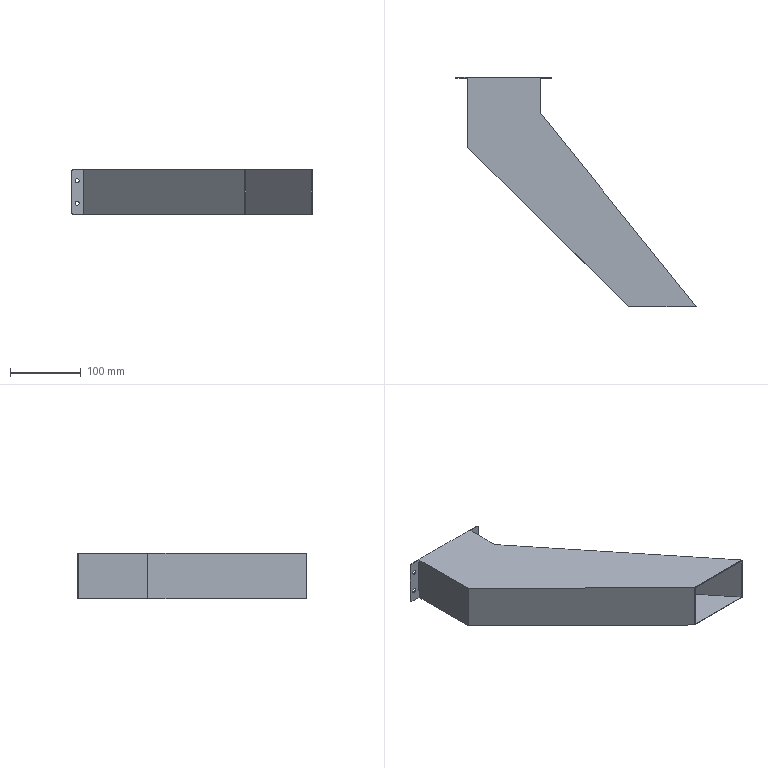Part | NX | 1 solid | 30 faces | box 340.79 x 325 x 65 mm | volume 130070 mm3 | plane 18 | cylinder 12 | commonest cylinder face diameters 6 x12
STEP:
#1=CARTESIAN_POINT('',(621.,-133.5,-79.28));
#2=VERTEX_POINT('',#1);
#3=CARTESIAN_POINT('',(607.526,-133.5,-79.28));
#4=VERTEX_POINT('',#3);
#5=CARTESIAN_POINT('',(556.,-133.5,-79.28));
#6=DIRECTION('',(-1.,0.,0.));
#7=VECTOR('',#6,1000.);
#8=LINE('',#5,#7);
#9=EDGE_CURVE('',#2,#4,#8,.T.);
#10=ORIENTED_EDGE('',*,*,#9,.T.);
#11=CARTESIAN_POINT('',(607.526,-133.5,-144.28));
#12=VERTEX_POINT('',#11);
#13=CARTESIAN_POINT('',(607.526,-133.5,-79.28));
#14=DIRECTION('',(0.,0.,-1.));
#15=VECTOR('',#14,1000.);
#16=LINE('',#13,#15);
#17=EDGE_CURVE('',#4,#12,#16,.T.);
#18=ORIENTED_EDGE('',*,*,#17,.T.);
#19=CARTESIAN_POINT('',(621.,-133.5,-144.28));
#20=VERTEX_POINT('',#19);
#21=CARTESIAN_POINT('',(556.,-133.5,-144.28));
#22=DIRECTION('',(-1.,0.,0.));
#23=VECTOR('',#22,1000.);
#24=LINE('',#21,#23);
#25=EDGE_CURVE('',#20,#12,#24,.T.);
#26=ORIENTED_EDGE('',*,*,#25,.F.);
#27=CARTESIAN_POINT('',(624.,-133.5,-141.28));
#28=VERTEX_POINT('',#27);
#29=CARTESIAN_POINT('',(621.,-133.5,-141.28));
#30=DIRECTION('',(0.,-1.,0.));
#31=DIRECTION('',(-1.,0.,0.));
#32=AXIS2_PLACEMENT_3D('',#29,#30,#31);
#33=CIRCLE('',#32,3.);
#34=EDGE_CURVE('',#20,#28,#33,.T.);
#35=ORIENTED_EDGE('',*,*,#34,.T.);
#36=CARTESIAN_POINT('',(624.,-133.5,-82.28));
#37=VERTEX_POINT('',#36);
#38=CARTESIAN_POINT('',(624.,-133.5,-79.28));
#39=DIRECTION('',(0.,0.,-1.));
#40=VECTOR('',#39,1000.);
#41=LINE('',#38,#40);
#42=EDGE_CURVE('',#37,#28,#41,.T.);
#43=ORIENTED_EDGE('',*,*,#42,.F.);
#44=CARTESIAN_POINT('',(621.,-133.5,-82.28));
#45=DIRECTION('',(0.,-1.,0.));
#46=DIRECTION('',(-1.,0.,0.));
#47=AXIS2_PLACEMENT_3D('',#44,#45,#46);
#48=CIRCLE('',#47,3.);
#49=EDGE_CURVE('',#37,#2,#48,.T.);
#50=ORIENTED_EDGE('',*,*,#49,.T.);
#51=EDGE_LOOP('',(#10,#18,#26,#35,#43,#50));
#52=FACE_BOUND('',#51,.T.);
#53=CARTESIAN_POINT('',(619.5,-133.5,-96.03));
#54=VERTEX_POINT('',#53);
#55=CARTESIAN_POINT('',(613.5,-133.5,-96.03));
#56=VERTEX_POINT('',#55);
#57=CARTESIAN_POINT('',(616.5,-133.5,-96.03));
#58=DIRECTION('',(0.,-1.,0.));
#59=DIRECTION('',(-1.,0.,0.));
#60=AXIS2_PLACEMENT_3D('',#57,#58,#59);
#61=CIRCLE('',#60,3.);
#62=EDGE_CURVE('',#54,#56,#61,.T.);
#63=ORIENTED_EDGE('',*,*,#62,.F.);
#64=CARTESIAN_POINT('',(616.5,-133.5,-96.03));
#65=DIRECTION('',(0.,-1.,0.));
#66=DIRECTION('',(-1.,0.,0.));
#67=AXIS2_PLACEMENT_3D('',#64,#65,#66);
#68=CIRCLE('',#67,3.);
#69=EDGE_CURVE('',#56,#54,#68,.T.);
#70=ORIENTED_EDGE('',*,*,#69,.F.);
#71=EDGE_LOOP('',(#63,#70));
#72=FACE_BOUND('',#71,.T.);
#73=CARTESIAN_POINT('',(619.5,-133.5,-127.53));
#74=VERTEX_POINT('',#73);
#75=CARTESIAN_POINT('',(613.5,-133.5,-127.53));
#76=VERTEX_POINT('',#75);
#77=CARTESIAN_POINT('',(616.5,-133.5,-127.53));
#78=DIRECTION('',(0.,-1.,0.));
#79=DIRECTION('',(-1.,0.,0.));
#80=AXIS2_PLACEMENT_3D('',#77,#78,#79);
#81=CIRCLE('',#80,3.);
#82=EDGE_CURVE('',#74,#76,#81,.T.);
#83=ORIENTED_EDGE('',*,*,#82,.F.);
#84=CARTESIAN_POINT('',(616.5,-133.5,-127.53));
#85=DIRECTION('',(0.,-1.,0.));
#86=DIRECTION('',(-1.,0.,0.));
#87=AXIS2_PLACEMENT_3D('',#84,#85,#86);
#88=CIRCLE('',#87,3.);
#89=EDGE_CURVE('',#76,#74,#88,.T.);
#90=ORIENTED_EDGE('',*,*,#89,.F.);
#91=EDGE_LOOP('',(#83,#90));
#92=FACE_BOUND('',#91,.T.);
#93=CARTESIAN_POINT('',(607.526,-133.5,-79.28));
#94=DIRECTION('',(0.,-1.,0.));
#95=DIRECTION('',(0.,0.,-1.));
#96=AXIS2_PLACEMENT_3D('',#93,#94,#95);
#97=PLANE('',#96);
#98=ADVANCED_FACE('',(#52,#72,#92),#97,.T.);
#99=CARTESIAN_POINT('',(607.526,-182.5,-79.28));
#100=VERTEX_POINT('',#99);
#101=CARTESIAN_POINT('',(607.526,-132.5,-79.28));
#102=DIRECTION('',(0.,-1.,0.));
#103=VECTOR('',#102,1000.);
#104=LINE('',#101,#103);
#105=EDGE_CURVE('',#4,#100,#104,.T.);
#106=ORIENTED_EDGE('',*,*,#105,.T.);
#107=CARTESIAN_POINT('',(607.526,-182.5,-144.28));
#108=VERTEX_POINT('',#107);
#109=CARTESIAN_POINT('',(607.526,-182.5,-79.28));
#110=DIRECTION('',(0.,0.,-1.));
#111=VECTOR('',#110,1000.);
#112=LINE('',#109,#111);
#113=EDGE_CURVE('',#100,#108,#112,.T.);
#114=ORIENTED_EDGE('',*,*,#113,.T.);
#115=CARTESIAN_POINT('',(607.526,-132.5,-144.28));
#116=DIRECTION('',(0.,-1.,0.));
#117=VECTOR('',#116,1000.);
#118=LINE('',#115,#117);
#119=EDGE_CURVE('',#12,#108,#118,.T.);
#120=ORIENTED_EDGE('',*,*,#119,.F.);
#121=ORIENTED_EDGE('',*,*,#17,.F.);
#122=EDGE_LOOP('',(#106,#114,#120,#121));
#123=FACE_BOUND('',#122,.T.);
#124=CARTESIAN_POINT('',(607.526,-182.5,-79.28));
#125=DIRECTION('',(1.,0.,0.));
#126=DIRECTION('',(0.,1.,0.));
#127=AXIS2_PLACEMENT_3D('',#124,#125,#126);
#128=PLANE('',#127);
#129=ADVANCED_FACE('',(#123),#128,.T.);
#130=CARTESIAN_POINT('',(828.79,-457.5,-79.28));
#131=VERTEX_POINT('',#130);
#132=CARTESIAN_POINT('',(466.156,-6.797,-79.28));
#133=DIRECTION('',(0.6269,-0.7791,0.));
#134=VECTOR('',#133,1000.);
#135=LINE('',#132,#134);
#136=EDGE_CURVE('',#100,#131,#135,.T.);
#137=ORIENTED_EDGE('',*,*,#136,.T.);
#138=CARTESIAN_POINT('',(828.79,-457.5,-144.28));
#139=VERTEX_POINT('',#138);
#140=CARTESIAN_POINT('',(828.79,-457.5,-79.28));
#141=DIRECTION('',(0.,0.,-1.));
#142=VECTOR('',#141,1000.);
#143=LINE('',#140,#142);
#144=EDGE_CURVE('',#131,#139,#143,.T.);
#145=ORIENTED_EDGE('',*,*,#144,.T.);
#146=CARTESIAN_POINT('',(466.156,-6.797,-144.28));
#147=DIRECTION('',(0.6269,-0.7791,0.));
#148=VECTOR('',#147,1000.);
#149=LINE('',#146,#148);
#150=EDGE_CURVE('',#108,#139,#149,.T.);
#151=ORIENTED_EDGE('',*,*,#150,.F.);
#152=ORIENTED_EDGE('',*,*,#113,.F.);
#153=EDGE_LOOP('',(#137,#145,#151,#152));
#154=FACE_BOUND('',#153,.T.);
#155=CARTESIAN_POINT('',(828.79,-457.5,-79.28));
#156=DIRECTION('',(0.7791,0.6269,0.));
#157=DIRECTION('',(0.,0.,-1.));
#158=AXIS2_PLACEMENT_3D('',#155,#156,#157);
#159=PLANE('',#158);
#160=ADVANCED_FACE('',(#154),#159,.T.);
#161=CARTESIAN_POINT('',(733.247,-457.5,-79.28));
#162=VERTEX_POINT('',#161);
#163=CARTESIAN_POINT('',(564.98,-457.5,-79.28));
#164=DIRECTION('',(1.,0.,0.));
#165=VECTOR('',#164,1000.);
#166=LINE('',#163,#165);
#167=EDGE_CURVE('',#162,#131,#166,.T.);
#168=ORIENTED_EDGE('',*,*,#167,.F.);
#169=CARTESIAN_POINT('',(733.247,-457.5,-144.28));
#170=VERTEX_POINT('',#169);
#171=CARTESIAN_POINT('',(733.247,-457.5,-79.28));
#172=DIRECTION('',(0.,0.,-1.));
#173=VECTOR('',#172,1000.);
#174=LINE('',#171,#173);
#175=EDGE_CURVE('',#162,#170,#174,.T.);
#176=ORIENTED_EDGE('',*,*,#175,.T.);
#177=CARTESIAN_POINT('',(564.98,-457.5,-144.28));
#178=DIRECTION('',(1.,0.,0.));
#179=VECTOR('',#178,1000.);
#180=LINE('',#177,#179);
#181=EDGE_CURVE('',#170,#139,#180,.T.);
#182=ORIENTED_EDGE('',*,*,#181,.T.);
#183=ORIENTED_EDGE('',*,*,#144,.F.);
#184=EDGE_LOOP('',(#168,#176,#182,#183));
#185=FACE_BOUND('',#184,.T.);
#186=CARTESIAN_POINT('',(734.672,-457.5,-80.28));
#187=VERTEX_POINT('',#186);
#188=CARTESIAN_POINT('',(734.672,-457.5,-143.28));
#189=VERTEX_POINT('',#188);
#190=CARTESIAN_POINT('',(734.672,-457.5,-79.28));
#191=DIRECTION('',(0.,0.,-1.));
#192=VECTOR('',#191,1000.);
#193=LINE('',#190,#192);
#194=EDGE_CURVE('',#187,#189,#193,.T.);
#195=ORIENTED_EDGE('',*,*,#194,.F.);
#196=CARTESIAN_POINT('',(827.507,-457.5,-80.28));
#197=VERTEX_POINT('',#196);
#198=CARTESIAN_POINT('',(1140.033,-457.5,-80.28));
#199=DIRECTION('',(-1.,0.,0.));
#200=VECTOR('',#199,1000.);
#201=LINE('',#198,#200);
#202=EDGE_CURVE('',#197,#187,#201,.T.);
#203=ORIENTED_EDGE('',*,*,#202,.F.);
#204=CARTESIAN_POINT('',(827.507,-457.5,-143.28));
#205=VERTEX_POINT('',#204);
#206=CARTESIAN_POINT('',(827.507,-457.5,-79.28));
#207=DIRECTION('',(0.,0.,1.));
#208=VECTOR('',#207,1000.);
#209=LINE('',#206,#208);
#210=EDGE_CURVE('',#205,#197,#209,.T.);
#211=ORIENTED_EDGE('',*,*,#210,.F.);
#212=CARTESIAN_POINT('',(1140.033,-457.5,-143.28));
#213=DIRECTION('',(-1.,0.,0.));
#214=VECTOR('',#213,1000.);
#215=LINE('',#212,#214);
#216=EDGE_CURVE('',#205,#189,#215,.T.);
#217=ORIENTED_EDGE('',*,*,#216,.T.);
#218=EDGE_LOOP('',(#195,#203,#211,#217));
#219=FACE_BOUND('',#218,.T.);
#220=CARTESIAN_POINT('',(733.247,-457.5,-79.28));
#221=DIRECTION('',(0.,-1.,0.));
#222=DIRECTION('',(0.,0.,-1.));
#223=AXIS2_PLACEMENT_3D('',#220,#221,#222);
#224=PLANE('',#223);
#225=ADVANCED_FACE('',(#185,#219),#224,.T.);
#226=CARTESIAN_POINT('',(505.,-232.5,-79.28));
#227=VERTEX_POINT('',#226);
#228=CARTESIAN_POINT('',(564.98,-291.626,-79.28));
#229=DIRECTION('',(-0.7122,0.702,0.));
#230=VECTOR('',#229,1000.);
#231=LINE('',#228,#230);
#232=EDGE_CURVE('',#162,#227,#231,.T.);
#233=ORIENTED_EDGE('',*,*,#232,.T.);
#234=CARTESIAN_POINT('',(505.,-232.5,-144.28));
#235=VERTEX_POINT('',#234);
#236=CARTESIAN_POINT('',(505.,-232.5,-79.28));
#237=DIRECTION('',(0.,0.,-1.));
#238=VECTOR('',#237,1000.);
#239=LINE('',#236,#238);
#240=EDGE_CURVE('',#227,#235,#239,.T.);
#241=ORIENTED_EDGE('',*,*,#240,.T.);
#242=CARTESIAN_POINT('',(564.98,-291.626,-144.28));
#243=DIRECTION('',(-0.7122,0.702,0.));
#244=VECTOR('',#243,1000.);
#245=LINE('',#242,#244);
#246=EDGE_CURVE('',#170,#235,#245,.T.);
#247=ORIENTED_EDGE('',*,*,#246,.F.);
#248=ORIENTED_EDGE('',*,*,#175,.F.);
#249=EDGE_LOOP('',(#233,#241,#247,#248));
#250=FACE_BOUND('',#249,.T.);
#251=CARTESIAN_POINT('',(505.,-232.5,-79.28));
#252=DIRECTION('',(-0.702,-0.7122,0.));
#253=DIRECTION('',(-0.7122,0.702,0.));
#254=AXIS2_PLACEMENT_3D('',#251,#252,#253);
#255=PLANE('',#254);
#256=ADVANCED_FACE('',(#250),#255,.T.);
#257=CARTESIAN_POINT('',(505.,-133.5,-79.28));
#258=VERTEX_POINT('',#257);
#259=CARTESIAN_POINT('',(505.,-132.5,-79.28));
#260=DIRECTION('',(0.,-1.,0.));
#261=VECTOR('',#260,1000.);
#262=LINE('',#259,#261);
#263=EDGE_CURVE('',#258,#227,#262,.T.);
#264=ORIENTED_EDGE('',*,*,#263,.F.);
#265=CARTESIAN_POINT('',(505.,-133.5,-144.28));
#266=VERTEX_POINT('',#265);
#267=CARTESIAN_POINT('',(505.,-133.5,-79.28));
#268=DIRECTION('',(0.,0.,-1.));
#269=VECTOR('',#268,1000.);
#270=LINE('',#267,#269);
#271=EDGE_CURVE('',#258,#266,#270,.T.);
#272=ORIENTED_EDGE('',*,*,#271,.T.);
#273=CARTESIAN_POINT('',(505.,-132.5,-144.28));
#274=DIRECTION('',(0.,-1.,0.));
#275=VECTOR('',#274,1000.);
#276=LINE('',#273,#275);
#277=EDGE_CURVE('',#266,#235,#276,.T.);
#278=ORIENTED_EDGE('',*,*,#277,.T.);
#279=ORIENTED_EDGE('',*,*,#240,.F.);
#280=EDGE_LOOP('',(#264,#272,#278,#279));
#281=FACE_BOUND('',#280,.T.);
#282=CARTESIAN_POINT('',(505.,-133.5,-79.28));
#283=DIRECTION('',(-1.,0.,0.));
#284=DIRECTION('',(0.,1.,0.));
#285=AXIS2_PLACEMENT_3D('',#282,#283,#284);
#286=PLANE('',#285);
#287=ADVANCED_FACE('',(#281),#286,.T.);
#288=CARTESIAN_POINT('',(491.,-133.5,-79.28));
#289=VERTEX_POINT('',#288);
#290=CARTESIAN_POINT('',(556.,-133.5,-79.28));
#291=DIRECTION('',(-1.,0.,0.));
#292=VECTOR('',#291,1000.);
#293=LINE('',#290,#292);
#294=EDGE_CURVE('',#258,#289,#293,.T.);
#295=ORIENTED_EDGE('',*,*,#294,.T.);
#296=CARTESIAN_POINT('',(488.,-133.5,-82.28));
#297=VERTEX_POINT('',#296);
#298=CARTESIAN_POINT('',(491.,-133.5,-82.28));
#299=DIRECTION('',(0.,-1.,0.));
#300=DIRECTION('',(-1.,0.,0.));
#301=AXIS2_PLACEMENT_3D('',#298,#299,#300);
#302=CIRCLE('',#301,3.);
#303=EDGE_CURVE('',#289,#297,#302,.T.);
#304=ORIENTED_EDGE('',*,*,#303,.T.);
#305=CARTESIAN_POINT('',(488.,-133.5,-141.28));
#306=VERTEX_POINT('',#305);
#307=CARTESIAN_POINT('',(488.,-133.5,-79.28));
#308=DIRECTION('',(0.,0.,-1.));
#309=VECTOR('',#308,1000.);
#310=LINE('',#307,#309);
#311=EDGE_CURVE('',#297,#306,#310,.T.);
#312=ORIENTED_EDGE('',*,*,#311,.T.);
#313=CARTESIAN_POINT('',(491.,-133.5,-144.28));
#314=VERTEX_POINT('',#313);
#315=CARTESIAN_POINT('',(491.,-133.5,-141.28));
#316=DIRECTION('',(0.,-1.,0.));
#317=DIRECTION('',(-1.,0.,0.));
#318=AXIS2_PLACEMENT_3D('',#315,#316,#317);
#319=CIRCLE('',#318,3.);
#320=EDGE_CURVE('',#306,#314,#319,.T.);
#321=ORIENTED_EDGE('',*,*,#320,.T.);
#322=CARTESIAN_POINT('',(556.,-133.5,-144.28));
#323=DIRECTION('',(-1.,0.,0.));
#324=VECTOR('',#323,1000.);
#325=LINE('',#322,#324);
#326=EDGE_CURVE('',#266,#314,#325,.T.);
#327=ORIENTED_EDGE('',*,*,#326,.F.);
#328=ORIENTED_EDGE('',*,*,#271,.F.);
#329=EDGE_LOOP('',(#295,#304,#312,#321,#327,#328));
#330=FACE_BOUND('',#329,.T.);
#331=CARTESIAN_POINT('',(498.5,-133.5,-96.03));
#332=VERTEX_POINT('',#331);
#333=CARTESIAN_POINT('',(492.5,-133.5,-96.03));
#334=VERTEX_POINT('',#333);
#335=CARTESIAN_POINT('',(495.5,-133.5,-96.03));
#336=DIRECTION('',(0.,-1.,0.));
#337=DIRECTION('',(-1.,0.,0.));
#338=AXIS2_PLACEMENT_3D('',#335,#336,#337);
#339=CIRCLE('',#338,3.);
#340=EDGE_CURVE('',#332,#334,#339,.T.);
#341=ORIENTED_EDGE('',*,*,#340,.F.);
#342=CARTESIAN_POINT('',(495.5,-133.5,-96.03));
#343=DIRECTION('',(0.,-1.,0.));
#344=DIRECTION('',(-1.,0.,0.));
#345=AXIS2_PLACEMENT_3D('',#342,#343,#344);
#346=CIRCLE('',#345,3.);
#347=EDGE_CURVE('',#334,#332,#346,.T.);
#348=ORIENTED_EDGE('',*,*,#347,.F.);
#349=EDGE_LOOP('',(#341,#348));
#350=FACE_BOUND('',#349,.T.);
#351=CARTESIAN_POINT('',(498.5,-133.5,-127.53));
#352=VERTEX_POINT('',#351);
#353=CARTESIAN_POINT('',(492.5,-133.5,-127.53));
#354=VERTEX_POINT('',#353);
#355=CARTESIAN_POINT('',(495.5,-133.5,-127.53));
#356=DIRECTION('',(0.,-1.,0.));
#357=DIRECTION('',(-1.,0.,0.));
#358=AXIS2_PLACEMENT_3D('',#355,#356,#357);
#359=CIRCLE('',#358,3.);
#360=EDGE_CURVE('',#352,#354,#359,.T.);
#361=ORIENTED_EDGE('',*,*,#360,.F.);
#362=CARTESIAN_POINT('',(495.5,-133.5,-127.53));
#363=DIRECTION('',(0.,-1.,0.));
#364=DIRECTION('',(-1.,0.,0.));
#365=AXIS2_PLACEMENT_3D('',#362,#363,#364);
#366=CIRCLE('',#365,3.);
#367=EDGE_CURVE('',#354,#352,#366,.T.);
#368=ORIENTED_EDGE('',*,*,#367,.F.);
#369=EDGE_LOOP('',(#361,#368));
#370=FACE_BOUND('',#369,.T.);
#371=CARTESIAN_POINT('',(488.,-133.5,-79.28));
#372=DIRECTION('',(0.,-1.,0.));
#373=DIRECTION('',(0.,0.,-1.));
#374=AXIS2_PLACEMENT_3D('',#371,#372,#373);
#375=PLANE('',#374);
#376=ADVANCED_FACE('',(#330,#350,#370),#375,.T.);
#377=CARTESIAN_POINT('',(488.,-132.5,-82.28));
#378=VERTEX_POINT('',#377);
#379=CARTESIAN_POINT('',(488.,-72.544,-82.28));
#380=DIRECTION('',(0.,-1.,0.));
#381=VECTOR('',#380,1000.);
#382=LINE('',#379,#381);
#383=EDGE_CURVE('',#378,#297,#382,.T.);
#384=ORIENTED_EDGE('',*,*,#383,.F.);
#385=CARTESIAN_POINT('',(488.,-132.5,-141.28));
#386=VERTEX_POINT('',#385);
#387=CARTESIAN_POINT('',(488.,-132.5,-79.28));
#388=DIRECTION('',(0.,0.,-1.));
#389=VECTOR('',#388,1000.);
#390=LINE('',#387,#389);
#391=EDGE_CURVE('',#378,#386,#390,.T.);
#392=ORIENTED_EDGE('',*,*,#391,.T.);
#393=CARTESIAN_POINT('',(488.,-72.544,-141.28));
#394=DIRECTION('',(0.,-1.,0.));
#395=VECTOR('',#394,1000.);
#396=LINE('',#393,#395);
#397=EDGE_CURVE('',#386,#306,#396,.T.);
#398=ORIENTED_EDGE('',*,*,#397,.T.);
#399=ORIENTED_EDGE('',*,*,#311,.F.);
#400=EDGE_LOOP('',(#384,#392,#398,#399));
#401=FACE_BOUND('',#400,.T.);
#402=CARTESIAN_POINT('',(488.,-132.5,-79.28));
#403=DIRECTION('',(-1.,0.,0.));
#404=DIRECTION('',(0.,0.,1.));
#405=AXIS2_PLACEMENT_3D('',#402,#403,#404);
#406=PLANE('',#405);
#407=ADVANCED_FACE('',(#401),#406,.T.);
#408=CARTESIAN_POINT('',(621.,-132.5,-79.28));
#409=VERTEX_POINT('',#408);
#410=CARTESIAN_POINT('',(491.,-132.5,-79.28));
#411=VERTEX_POINT('',#410);
#412=CARTESIAN_POINT('',(556.,-132.5,-79.28));
#413=DIRECTION('',(-1.,0.,0.));
#414=VECTOR('',#413,1000.);
#415=LINE('',#412,#414);
#416=EDGE_CURVE('',#409,#411,#415,.T.);
#417=ORIENTED_EDGE('',*,*,#416,.F.);
#418=CARTESIAN_POINT('',(624.,-132.5,-82.28));
#419=VERTEX_POINT('',#418);
#420=CARTESIAN_POINT('',(621.,-132.5,-82.28));
#421=DIRECTION('',(0.,-1.,0.));
#422=DIRECTION('',(-1.,0.,0.));
#423=AXIS2_PLACEMENT_3D('',#420,#421,#422);
#424=CIRCLE('',#423,3.);
#425=EDGE_CURVE('',#419,#409,#424,.T.);
#426=ORIENTED_EDGE('',*,*,#425,.F.);
#427=CARTESIAN_POINT('',(624.,-132.5,-141.28));
#428=VERTEX_POINT('',#427);
#429=CARTESIAN_POINT('',(624.,-132.5,-79.28));
#430=DIRECTION('',(0.,0.,-1.));
#431=VECTOR('',#430,1000.);
#432=LINE('',#429,#431);
#433=EDGE_CURVE('',#419,#428,#432,.T.);
#434=ORIENTED_EDGE('',*,*,#433,.T.);
#435=CARTESIAN_POINT('',(621.,-132.5,-144.28));
#436=VERTEX_POINT('',#435);
#437=CARTESIAN_POINT('',(621.,-132.5,-141.28));
#438=DIRECTION('',(0.,-1.,0.));
#439=DIRECTION('',(-1.,0.,0.));
#440=AXIS2_PLACEMENT_3D('',#437,#438,#439);
#441=CIRCLE('',#440,3.);
#442=EDGE_CURVE('',#436,#428,#441,.T.);
#443=ORIENTED_EDGE('',*,*,#442,.F.);
#444=CARTESIAN_POINT('',(491.,-132.5,-144.28));
#445=VERTEX_POINT('',#444);
#446=CARTESIAN_POINT('',(556.,-132.5,-144.28));
#447=DIRECTION('',(-1.,0.,0.));
#448=VECTOR('',#447,1000.);
#449=LINE('',#446,#448);
#450=EDGE_CURVE('',#436,#445,#449,.T.);
#451=ORIENTED_EDGE('',*,*,#450,.T.);
#452=CARTESIAN_POINT('',(491.,-132.5,-141.28));
#453=DIRECTION('',(0.,-1.,0.));
#454=DIRECTION('',(-1.,0.,0.));
#455=AXIS2_PLACEMENT_3D('',#452,#453,#454);
#456=CIRCLE('',#455,3.);
#457=EDGE_CURVE('',#386,#445,#456,.T.);
#458=ORIENTED_EDGE('',*,*,#457,.F.);
#459=ORIENTED_EDGE('',*,*,#391,.F.);
#460=CARTESIAN_POINT('',(491.,-132.5,-82.28));
#461=DIRECTION('',(0.,-1.,0.));
#462=DIRECTION('',(-1.,0.,0.));
#463=AXIS2_PLACEMENT_3D('',#460,#461,#462);
#464=CIRCLE('',#463,3.);
#465=EDGE_CURVE('',#411,#378,#464,.T.);
#466=ORIENTED_EDGE('',*,*,#465,.F.);
#467=EDGE_LOOP('',(#417,#426,#434,#443,#451,#458,#459,#466));
#468=FACE_BOUND('',#467,.T.);
#469=CARTESIAN_POINT('',(506.,-132.5,-143.28));
#470=VERTEX_POINT('',#469);
#471=CARTESIAN_POINT('',(506.,-132.5,-80.28));
#472=VERTEX_POINT('',#471);
#473=CARTESIAN_POINT('',(506.,-132.5,-79.28));
#474=DIRECTION('',(0.,0.,1.));
#475=VECTOR('',#474,1000.);
#476=LINE('',#473,#475);
#477=EDGE_CURVE('',#470,#472,#476,.T.);
#478=ORIENTED_EDGE('',*,*,#477,.F.);
#479=CARTESIAN_POINT('',(606.526,-132.5,-143.28));
#480=VERTEX_POINT('',#479);
#481=CARTESIAN_POINT('',(1140.033,-132.5,-143.28));
#482=DIRECTION('',(-1.,0.,0.));
#483=VECTOR('',#482,1000.);
#484=LINE('',#481,#483);
#485=EDGE_CURVE('',#480,#470,#484,.T.);
#486=ORIENTED_EDGE('',*,*,#485,.F.);
#487=CARTESIAN_POINT('',(606.526,-132.5,-80.28));
#488=VERTEX_POINT('',#487);
#489=CARTESIAN_POINT('',(606.526,-132.5,-79.28));
#490=DIRECTION('',(0.,0.,-1.));
#491=VECTOR('',#490,1000.);
#492=LINE('',#489,#491);
#493=EDGE_CURVE('',#488,#480,#492,.T.);
#494=ORIENTED_EDGE('',*,*,#493,.F.);
#495=CARTESIAN_POINT('',(1140.033,-132.5,-80.28));
#496=DIRECTION('',(1.,0.,0.));
#497=VECTOR('',#496,1000.);
#498=LINE('',#495,#497);
#499=EDGE_CURVE('',#472,#488,#498,.T.);
#500=ORIENTED_EDGE('',*,*,#499,.F.);
#501=EDGE_LOOP('',(#478,#486,#494,#500));
#502=FACE_BOUND('',#501,.T.);
#503=CARTESIAN_POINT('',(619.5,-132.5,-96.03));
#504=VERTEX_POINT('',#503);
#505=CARTESIAN_POINT('',(613.5,-132.5,-96.03));
#506=VERTEX_POINT('',#505);
#507=CARTESIAN_POINT('',(616.5,-132.5,-96.03));
#508=DIRECTION('',(0.,-1.,0.));
#509=DIRECTION('',(-1.,0.,0.));
#510=AXIS2_PLACEMENT_3D('',#507,#508,#509);
#511=CIRCLE('',#510,3.);
#512=EDGE_CURVE('',#504,#506,#511,.T.);
#513=ORIENTED_EDGE('',*,*,#512,.T.);
#514=CARTESIAN_POINT('',(616.5,-132.5,-96.03));
#515=DIRECTION('',(0.,-1.,0.));
#516=DIRECTION('',(-1.,0.,0.));
#517=AXIS2_PLACEMENT_3D('',#514,#515,#516);
#518=CIRCLE('',#517,3.);
#519=EDGE_CURVE('',#506,#504,#518,.T.);
#520=ORIENTED_EDGE('',*,*,#519,.T.);
#521=EDGE_LOOP('',(#513,#520));
#522=FACE_BOUND('',#521,.T.);
#523=CARTESIAN_POINT('',(498.5,-132.5,-127.53));
#524=VERTEX_POINT('',#523);
#525=CARTESIAN_POINT('',(492.5,-132.5,-127.53));
#526=VERTEX_POINT('',#525);
#527=CARTESIAN_POINT('',(495.5,-132.5,-127.53));
#528=DIRECTION('',(0.,-1.,0.));
#529=DIRECTION('',(-1.,0.,0.));
#530=AXIS2_PLACEMENT_3D('',#527,#528,#529);
#531=CIRCLE('',#530,3.);
#532=EDGE_CURVE('',#524,#526,#531,.T.);
#533=ORIENTED_EDGE('',*,*,#532,.T.);
#534=CARTESIAN_POINT('',(495.5,-132.5,-127.53));
#535=DIRECTION('',(0.,-1.,0.));
#536=DIRECTION('',(-1.,0.,0.));
#537=AXIS2_PLACEMENT_3D('',#534,#535,#536);
#538=CIRCLE('',#537,3.);
#539=EDGE_CURVE('',#526,#524,#538,.T.);
#540=ORIENTED_EDGE('',*,*,#539,.T.);
#541=EDGE_LOOP('',(#533,#540));
#542=FACE_BOUND('',#541,.T.);
#543=CARTESIAN_POINT('',(619.5,-132.5,-127.53));
#544=VERTEX_POINT('',#543);
#545=CARTESIAN_POINT('',(613.5,-132.5,-127.53));
#546=VERTEX_POINT('',#545);
#547=CARTESIAN_POINT('',(616.5,-132.5,-127.53));
#548=DIRECTION('',(0.,-1.,0.));
#549=DIRECTION('',(-1.,0.,0.));
#550=AXIS2_PLACEMENT_3D('',#547,#548,#549);
#551=CIRCLE('',#550,3.);
#552=EDGE_CURVE('',#544,#546,#551,.T.);
#553=ORIENTED_EDGE('',*,*,#552,.T.);
#554=CARTESIAN_POINT('',(616.5,-132.5,-127.53));
#555=DIRECTION('',(0.,-1.,0.));
#556=DIRECTION('',(-1.,0.,0.));
#557=AXIS2_PLACEMENT_3D('',#554,#555,#556);
#558=CIRCLE('',#557,3.);
#559=EDGE_CURVE('',#546,#544,#558,.T.);
#560=ORIENTED_EDGE('',*,*,#559,.T.);
#561=EDGE_LOOP('',(#553,#560));
#562=FACE_BOUND('',#561,.T.);
#563=CARTESIAN_POINT('',(498.5,-132.5,-96.03));
#564=VERTEX_POINT('',#563);
#565=CARTESIAN_POINT('',(492.5,-132.5,-96.03));
#566=VERTEX_POINT('',#565);
#567=CARTESIAN_POINT('',(495.5,-132.5,-96.03));
#568=DIRECTION('',(0.,-1.,0.));
#569=DIRECTION('',(-1.,0.,0.));
#570=AXIS2_PLACEMENT_3D('',#567,#568,#569);
#571=CIRCLE('',#570,3.);
#572=EDGE_CURVE('',#564,#566,#571,.T.);
#573=ORIENTED_EDGE('',*,*,#572,.T.);
#574=CARTESIAN_POINT('',(495.5,-132.5,-96.03));
#575=DIRECTION('',(0.,-1.,0.));
#576=DIRECTION('',(-1.,0.,0.));
#577=AXIS2_PLACEMENT_3D('',#574,#575,#576);
#578=CIRCLE('',#577,3.);
#579=EDGE_CURVE('',#566,#564,#578,.T.);
#580=ORIENTED_EDGE('',*,*,#579,.T.);
#581=EDGE_LOOP('',(#573,#580));
#582=FACE_BOUND('',#581,.T.);
#583=CARTESIAN_POINT('',(624.,-132.5,-79.28));
#584=DIRECTION('',(0.,1.,0.));
#585=DIRECTION('',(1.,0.,0.));
#586=AXIS2_PLACEMENT_3D('',#583,#584,#585);
#587=PLANE('',#586);
#588=ADVANCED_FACE('',(#468,#502,#522,#542,#562,#582),#587,.T.);
#589=CARTESIAN_POINT('',(624.,-72.544,-82.28));
#590=DIRECTION('',(0.,-1.,0.));
#591=VECTOR('',#590,1000.);
#592=LINE('',#589,#591);
#593=EDGE_CURVE('',#419,#37,#592,.T.);
#594=ORIENTED_EDGE('',*,*,#593,.T.);
#595=ORIENTED_EDGE('',*,*,#42,.T.);
#596=CARTESIAN_POINT('',(624.,-72.544,-141.28));
#597=DIRECTION('',(0.,-1.,0.));
#598=VECTOR('',#597,1000.);
#599=LINE('',#596,#598);
#600=EDGE_CURVE('',#428,#28,#599,.T.);
#601=ORIENTED_EDGE('',*,*,#600,.F.);
#602=ORIENTED_EDGE('',*,*,#433,.F.);
#603=EDGE_LOOP('',(#594,#595,#601,#602));
#604=FACE_BOUND('',#603,.T.);
#605=CARTESIAN_POINT('',(624.,-133.5,-79.28));
#606=DIRECTION('',(1.,0.,0.));
#607=DIRECTION('',(0.,1.,0.));
#608=AXIS2_PLACEMENT_3D('',#605,#606,#607);
#609=PLANE('',#608);
#610=ADVANCED_FACE('',(#604),#609,.T.);
#611=CARTESIAN_POINT('',(606.526,-182.852,-80.28));
#612=VERTEX_POINT('',#611);
#613=CARTESIAN_POINT('',(606.526,-182.852,-143.28));
#614=VERTEX_POINT('',#613);
#615=CARTESIAN_POINT('',(606.526,-182.852,-79.28));
#616=DIRECTION('',(0.,0.,-1.));
#617=VECTOR('',#616,1000.);
#618=LINE('',#615,#617);
#619=EDGE_CURVE('',#612,#614,#618,.T.);
#620=ORIENTED_EDGE('',*,*,#619,.T.);
#621=CARTESIAN_POINT('',(517.772,-72.544,-143.28));
#622=DIRECTION('',(0.6269,-0.7791,0.));
#623=VECTOR('',#622,1000.);
#624=LINE('',#621,#623);
#625=EDGE_CURVE('',#614,#205,#624,.T.);
#626=ORIENTED_EDGE('',*,*,#625,.T.);
#627=ORIENTED_EDGE('',*,*,#210,.T.);
#628=CARTESIAN_POINT('',(517.772,-72.544,-80.28));
#629=DIRECTION('',(0.6269,-0.7791,0.));
#630=VECTOR('',#629,1000.);
#631=LINE('',#628,#630);
#632=EDGE_CURVE('',#612,#197,#631,.T.);
#633=ORIENTED_EDGE('',*,*,#632,.F.);
#634=EDGE_LOOP('',(#620,#626,#627,#633));
#635=FACE_BOUND('',#634,.T.);
#636=CARTESIAN_POINT('',(828.011,-458.127,-79.28));
#637=DIRECTION('',(0.7791,0.6269,0.));
#638=DIRECTION('',(0.,0.,-1.));
#639=AXIS2_PLACEMENT_3D('',#636,#637,#638);
#640=PLANE('',#639);
#641=ADVANCED_FACE('',(#635),#640,.F.);
#642=CARTESIAN_POINT('',(606.526,-133.5,-80.28));
#643=DIRECTION('',(0.,1.,0.));
#644=VECTOR('',#643,1000.);
#645=LINE('',#642,#644);
#646=EDGE_CURVE('',#612,#488,#645,.T.);
#647=ORIENTED_EDGE('',*,*,#646,.T.);
#648=ORIENTED_EDGE('',*,*,#493,.T.);
#649=CARTESIAN_POINT('',(606.526,-72.544,-143.28));
#650=DIRECTION('',(0.,-1.,0.));
#651=VECTOR('',#650,1000.);
#652=LINE('',#649,#651);
#653=EDGE_CURVE('',#480,#614,#652,.T.);
#654=ORIENTED_EDGE('',*,*,#653,.T.);
#655=ORIENTED_EDGE('',*,*,#619,.F.);
#656=EDGE_LOOP('',(#647,#648,#654,#655));
#657=FACE_BOUND('',#656,.T.);
#658=CARTESIAN_POINT('',(606.526,-182.5,-79.28));
#659=DIRECTION('',(1.,0.,0.));
#660=DIRECTION('',(0.,1.,0.));
#661=AXIS2_PLACEMENT_3D('',#658,#659,#660);
#662=PLANE('',#661);
#663=ADVANCED_FACE('',(#657),#662,.F.);
#664=CARTESIAN_POINT('',(506.,-232.082,-143.28));
#665=VERTEX_POINT('',#664);
#666=CARTESIAN_POINT('',(506.,-133.5,-143.28));
#667=DIRECTION('',(0.,1.,0.));
#668=VECTOR('',#667,1000.);
#669=LINE('',#666,#668);
#670=EDGE_CURVE('',#665,#470,#669,.T.);
#671=ORIENTED_EDGE('',*,*,#670,.T.);
#672=ORIENTED_EDGE('',*,*,#477,.T.);
#673=CARTESIAN_POINT('',(506.,-232.082,-80.28));
#674=VERTEX_POINT('',#673);
#675=CARTESIAN_POINT('',(506.,-133.5,-80.28));
#676=DIRECTION('',(0.,1.,0.));
#677=VECTOR('',#676,1000.);
#678=LINE('',#675,#677);
#679=EDGE_CURVE('',#674,#472,#678,.T.);
#680=ORIENTED_EDGE('',*,*,#679,.F.);
#681=CARTESIAN_POINT('',(506.,-232.082,-79.28));
#682=DIRECTION('',(0.,0.,1.));
#683=VECTOR('',#682,1000.);
#684=LINE('',#681,#683);
#685=EDGE_CURVE('',#665,#674,#684,.T.);
#686=ORIENTED_EDGE('',*,*,#685,.F.);
#687=EDGE_LOOP('',(#671,#672,#680,#686));
#688=FACE_BOUND('',#687,.T.);
#689=CARTESIAN_POINT('',(506.,-133.5,-79.28));
#690=DIRECTION('',(-1.,0.,0.));
#691=DIRECTION('',(0.,1.,0.));
#692=AXIS2_PLACEMENT_3D('',#689,#690,#691);
#693=PLANE('',#692);
#694=ADVANCED_FACE('',(#688),#693,.F.);
#695=ORIENTED_EDGE('',*,*,#194,.T.);
#696=CARTESIAN_POINT('',(1140.033,-857.094,-143.28));
#697=DIRECTION('',(-0.7122,0.702,0.));
#698=VECTOR('',#697,1000.);
#699=LINE('',#696,#698);
#700=EDGE_CURVE('',#189,#665,#699,.T.);
#701=ORIENTED_EDGE('',*,*,#700,.T.);
#702=ORIENTED_EDGE('',*,*,#685,.T.);
#703=CARTESIAN_POINT('',(1140.033,-857.094,-80.28));
#704=DIRECTION('',(-0.7122,0.702,0.));
#705=VECTOR('',#704,1000.);
#706=LINE('',#703,#705);
#707=EDGE_CURVE('',#187,#674,#706,.T.);
#708=ORIENTED_EDGE('',*,*,#707,.F.);
#709=EDGE_LOOP('',(#695,#701,#702,#708));
#710=FACE_BOUND('',#709,.T.);
#711=CARTESIAN_POINT('',(505.702,-231.788,-79.28));
#712=DIRECTION('',(-0.702,-0.7122,0.));
#713=DIRECTION('',(-0.7122,0.702,0.));
#714=AXIS2_PLACEMENT_3D('',#711,#712,#713);
#715=PLANE('',#714);
#716=ADVANCED_FACE('',(#710),#715,.F.);
#717=ORIENTED_EDGE('',*,*,#679,.T.);
#718=ORIENTED_EDGE('',*,*,#499,.T.);
#719=ORIENTED_EDGE('',*,*,#646,.F.);
#720=ORIENTED_EDGE('',*,*,#632,.T.);
#721=ORIENTED_EDGE('',*,*,#202,.T.);
#722=ORIENTED_EDGE('',*,*,#707,.T.);
#723=EDGE_LOOP('',(#717,#718,#719,#720,#721,#722));
#724=FACE_BOUND('',#723,.T.);
#725=CARTESIAN_POINT('',(606.526,-133.5,-80.28));
#726=DIRECTION('',(0.,0.,1.));
#727=DIRECTION('',(1.,0.,0.));
#728=AXIS2_PLACEMENT_3D('',#725,#726,#727);
#729=PLANE('',#728);
#730=ADVANCED_FACE('',(#724),#729,.F.);
#731=ORIENTED_EDGE('',*,*,#670,.F.);
#732=ORIENTED_EDGE('',*,*,#700,.F.);
#733=ORIENTED_EDGE('',*,*,#216,.F.);
#734=ORIENTED_EDGE('',*,*,#625,.F.);
#735=ORIENTED_EDGE('',*,*,#653,.F.);
#736=ORIENTED_EDGE('',*,*,#485,.T.);
#737=EDGE_LOOP('',(#731,#732,#733,#734,#735,#736));
#738=FACE_BOUND('',#737,.T.);
#739=CARTESIAN_POINT('',(1140.033,-72.544,-143.28));
#740=DIRECTION('',(0.,0.,1.));
#741=DIRECTION('',(1.,0.,0.));
#742=AXIS2_PLACEMENT_3D('',#739,#740,#741);
#743=PLANE('',#742);
#744=ADVANCED_FACE('',(#738),#743,.T.);
#745=ORIENTED_EDGE('',*,*,#512,.F.);
#746=CARTESIAN_POINT('',(619.5,-132.5,-96.03));
#747=DIRECTION('',(0.,-1.,0.));
#748=VECTOR('',#747,1000.);
#749=LINE('',#746,#748);
#750=EDGE_CURVE('',#54,#504,#749,.F.);
#751=ORIENTED_EDGE('',*,*,#750,.F.);
#752=ORIENTED_EDGE('',*,*,#62,.T.);
#753=CARTESIAN_POINT('',(613.5,-132.5,-96.03));
#754=DIRECTION('',(0.,-1.,0.));
#755=VECTOR('',#754,1000.);
#756=LINE('',#753,#755);
#757=EDGE_CURVE('',#56,#506,#756,.F.);
#758=ORIENTED_EDGE('',*,*,#757,.T.);
#759=EDGE_LOOP('',(#745,#751,#752,#758));
#760=FACE_BOUND('',#759,.T.);
#761=CARTESIAN_POINT('',(616.5,-132.5,-96.03));
#762=DIRECTION('',(0.,-1.,0.));
#763=DIRECTION('',(-1.,0.,0.));
#764=AXIS2_PLACEMENT_3D('',#761,#762,#763);
#765=CYLINDRICAL_SURFACE('',#764,3.);
#766=ADVANCED_FACE('',(#760),#765,.F.);
#767=ORIENTED_EDGE('',*,*,#572,.F.);
#768=CARTESIAN_POINT('',(498.5,-132.5,-96.03));
#769=DIRECTION('',(0.,-1.,0.));
#770=VECTOR('',#769,1000.);
#771=LINE('',#768,#770);
#772=EDGE_CURVE('',#332,#564,#771,.F.);
#773=ORIENTED_EDGE('',*,*,#772,.F.);
#774=ORIENTED_EDGE('',*,*,#340,.T.);
#775=CARTESIAN_POINT('',(492.5,-132.5,-96.03));
#776=DIRECTION('',(0.,-1.,0.));
#777=VECTOR('',#776,1000.);
#778=LINE('',#775,#777);
#779=EDGE_CURVE('',#334,#566,#778,.F.);
#780=ORIENTED_EDGE('',*,*,#779,.T.);
#781=EDGE_LOOP('',(#767,#773,#774,#780));
#782=FACE_BOUND('',#781,.T.);
#783=CARTESIAN_POINT('',(495.5,-132.5,-96.03));
#784=DIRECTION('',(0.,-1.,0.));
#785=DIRECTION('',(-1.,0.,0.));
#786=AXIS2_PLACEMENT_3D('',#783,#784,#785);
#787=CYLINDRICAL_SURFACE('',#786,3.);
#788=ADVANCED_FACE('',(#782),#787,.F.);
#789=ORIENTED_EDGE('',*,*,#532,.F.);
#790=CARTESIAN_POINT('',(498.5,-132.5,-127.53));
#791=DIRECTION('',(0.,-1.,0.));
#792=VECTOR('',#791,1000.);
#793=LINE('',#790,#792);
#794=EDGE_CURVE('',#352,#524,#793,.F.);
#795=ORIENTED_EDGE('',*,*,#794,.F.);
#796=ORIENTED_EDGE('',*,*,#360,.T.);
#797=CARTESIAN_POINT('',(492.5,-132.5,-127.53));
#798=DIRECTION('',(0.,-1.,0.));
#799=VECTOR('',#798,1000.);
#800=LINE('',#797,#799);
#801=EDGE_CURVE('',#354,#526,#800,.F.);
#802=ORIENTED_EDGE('',*,*,#801,.T.);
#803=EDGE_LOOP('',(#789,#795,#796,#802));
#804=FACE_BOUND('',#803,.T.);
#805=CARTESIAN_POINT('',(495.5,-132.5,-127.53));
#806=DIRECTION('',(0.,-1.,0.));
#807=DIRECTION('',(-1.,0.,0.));
#808=AXIS2_PLACEMENT_3D('',#805,#806,#807);
#809=CYLINDRICAL_SURFACE('',#808,3.);
#810=ADVANCED_FACE('',(#804),#809,.F.);
#811=ORIENTED_EDGE('',*,*,#552,.F.);
#812=CARTESIAN_POINT('',(619.5,-132.5,-127.53));
#813=DIRECTION('',(0.,-1.,0.));
#814=VECTOR('',#813,1000.);
#815=LINE('',#812,#814);
#816=EDGE_CURVE('',#74,#544,#815,.F.);
#817=ORIENTED_EDGE('',*,*,#816,.F.);
#818=ORIENTED_EDGE('',*,*,#82,.T.);
#819=CARTESIAN_POINT('',(613.5,-132.5,-127.53));
#820=DIRECTION('',(0.,-1.,0.));
#821=VECTOR('',#820,1000.);
#822=LINE('',#819,#821);
#823=EDGE_CURVE('',#76,#546,#822,.F.);
#824=ORIENTED_EDGE('',*,*,#823,.T.);
#825=EDGE_LOOP('',(#811,#817,#818,#824));
#826=FACE_BOUND('',#825,.T.);
#827=CARTESIAN_POINT('',(616.5,-132.5,-127.53));
#828=DIRECTION('',(0.,-1.,0.));
#829=DIRECTION('',(-1.,0.,0.));
#830=AXIS2_PLACEMENT_3D('',#827,#828,#829);
#831=CYLINDRICAL_SURFACE('',#830,3.);
#832=ADVANCED_FACE('',(#826),#831,.F.);
#833=ORIENTED_EDGE('',*,*,#823,.F.);
#834=ORIENTED_EDGE('',*,*,#89,.T.);
#835=ORIENTED_EDGE('',*,*,#816,.T.);
#836=ORIENTED_EDGE('',*,*,#559,.F.);
#837=EDGE_LOOP('',(#833,#834,#835,#836));
#838=FACE_BOUND('',#837,.T.);
#839=CARTESIAN_POINT('',(616.5,-132.5,-127.53));
#840=DIRECTION('',(0.,-1.,0.));
#841=DIRECTION('',(-1.,0.,0.));
#842=AXIS2_PLACEMENT_3D('',#839,#840,#841);
#843=CYLINDRICAL_SURFACE('',#842,3.);
#844=ADVANCED_FACE('',(#838),#843,.F.);
#845=ORIENTED_EDGE('',*,*,#779,.F.);
#846=ORIENTED_EDGE('',*,*,#347,.T.);
#847=ORIENTED_EDGE('',*,*,#772,.T.);
#848=ORIENTED_EDGE('',*,*,#579,.F.);
#849=EDGE_LOOP('',(#845,#846,#847,#848));
#850=FACE_BOUND('',#849,.T.);
#851=CARTESIAN_POINT('',(495.5,-132.5,-96.03));
#852=DIRECTION('',(0.,-1.,0.));
#853=DIRECTION('',(-1.,0.,0.));
#854=AXIS2_PLACEMENT_3D('',#851,#852,#853);
#855=CYLINDRICAL_SURFACE('',#854,3.);
#856=ADVANCED_FACE('',(#850),#855,.F.);
#857=ORIENTED_EDGE('',*,*,#801,.F.);
#858=ORIENTED_EDGE('',*,*,#367,.T.);
#859=ORIENTED_EDGE('',*,*,#794,.T.);
#860=ORIENTED_EDGE('',*,*,#539,.F.);
#861=EDGE_LOOP('',(#857,#858,#859,#860));
#862=FACE_BOUND('',#861,.T.);
#863=CARTESIAN_POINT('',(495.5,-132.5,-127.53));
#864=DIRECTION('',(0.,-1.,0.));
#865=DIRECTION('',(-1.,0.,0.));
#866=AXIS2_PLACEMENT_3D('',#863,#864,#865);
#867=CYLINDRICAL_SURFACE('',#866,3.);
#868=ADVANCED_FACE('',(#862),#867,.F.);
#869=ORIENTED_EDGE('',*,*,#757,.F.);
#870=ORIENTED_EDGE('',*,*,#69,.T.);
#871=ORIENTED_EDGE('',*,*,#750,.T.);
#872=ORIENTED_EDGE('',*,*,#519,.F.);
#873=EDGE_LOOP('',(#869,#870,#871,#872));
#874=FACE_BOUND('',#873,.T.);
#875=CARTESIAN_POINT('',(616.5,-132.5,-96.03));
#876=DIRECTION('',(0.,-1.,0.));
#877=DIRECTION('',(-1.,0.,0.));
#878=AXIS2_PLACEMENT_3D('',#875,#876,#877);
#879=CYLINDRICAL_SURFACE('',#878,3.);
#880=ADVANCED_FACE('',(#874),#879,.F.);
#881=CARTESIAN_POINT('',(621.,-72.544,-144.28));
#882=DIRECTION('',(0.,-1.,0.));
#883=VECTOR('',#882,1000.);
#884=LINE('',#881,#883);
#885=EDGE_CURVE('',#436,#20,#884,.T.);
#886=ORIENTED_EDGE('',*,*,#885,.T.);
#887=ORIENTED_EDGE('',*,*,#25,.T.);
#888=ORIENTED_EDGE('',*,*,#119,.T.);
#889=ORIENTED_EDGE('',*,*,#150,.T.);
#890=ORIENTED_EDGE('',*,*,#181,.F.);
#891=ORIENTED_EDGE('',*,*,#246,.T.);
#892=ORIENTED_EDGE('',*,*,#277,.F.);
#893=ORIENTED_EDGE('',*,*,#326,.T.);
#894=CARTESIAN_POINT('',(491.,-72.544,-144.28));
#895=DIRECTION('',(0.,-1.,0.));
#896=VECTOR('',#895,1000.);
#897=LINE('',#894,#896);
#898=EDGE_CURVE('',#445,#314,#897,.T.);
#899=ORIENTED_EDGE('',*,*,#898,.F.);
#900=ORIENTED_EDGE('',*,*,#450,.F.);
#901=EDGE_LOOP('',(#886,#887,#888,#889,#890,#891,#892,#893,#899,#900));
#902=FACE_BOUND('',#901,.T.);
#903=CARTESIAN_POINT('',(1140.033,-72.544,-144.28));
#904=DIRECTION('',(0.,0.,1.));
#905=DIRECTION('',(1.,0.,0.));
#906=AXIS2_PLACEMENT_3D('',#903,#904,#905);
#907=PLANE('',#906);
#908=ADVANCED_FACE('',(#902),#907,.F.);
#909=ORIENTED_EDGE('',*,*,#898,.T.);
#910=ORIENTED_EDGE('',*,*,#320,.F.);
#911=ORIENTED_EDGE('',*,*,#397,.F.);
#912=ORIENTED_EDGE('',*,*,#457,.T.);
#913=EDGE_LOOP('',(#909,#910,#911,#912));
#914=FACE_BOUND('',#913,.T.);
#915=CARTESIAN_POINT('',(491.,-72.544,-141.28));
#916=DIRECTION('',(0.,-1.,0.));
#917=DIRECTION('',(-1.,0.,0.));
#918=AXIS2_PLACEMENT_3D('',#915,#916,#917);
#919=CYLINDRICAL_SURFACE('',#918,3.);
#920=ADVANCED_FACE('',(#914),#919,.T.);
#921=ORIENTED_EDGE('',*,*,#885,.F.);
#922=ORIENTED_EDGE('',*,*,#442,.T.);
#923=ORIENTED_EDGE('',*,*,#600,.T.);
#924=ORIENTED_EDGE('',*,*,#34,.F.);
#925=EDGE_LOOP('',(#921,#922,#923,#924));
#926=FACE_BOUND('',#925,.T.);
#927=CARTESIAN_POINT('',(621.,-72.544,-141.28));
#928=DIRECTION('',(0.,-1.,0.));
#929=DIRECTION('',(-1.,0.,0.));
#930=AXIS2_PLACEMENT_3D('',#927,#928,#929);
#931=CYLINDRICAL_SURFACE('',#930,3.);
#932=ADVANCED_FACE('',(#926),#931,.T.);
#933=CARTESIAN_POINT('',(621.,-72.544,-79.28));
#934=DIRECTION('',(0.,-1.,0.));
#935=VECTOR('',#934,1000.);
#936=LINE('',#933,#935);
#937=EDGE_CURVE('',#409,#2,#936,.T.);
#938=ORIENTED_EDGE('',*,*,#937,.F.);
#939=ORIENTED_EDGE('',*,*,#416,.T.);
#940=CARTESIAN_POINT('',(491.,-72.544,-79.28));
#941=DIRECTION('',(0.,-1.,0.));
#942=VECTOR('',#941,1000.);
#943=LINE('',#940,#942);
#944=EDGE_CURVE('',#411,#289,#943,.T.);
#945=ORIENTED_EDGE('',*,*,#944,.T.);
#946=ORIENTED_EDGE('',*,*,#294,.F.);
#947=ORIENTED_EDGE('',*,*,#263,.T.);
#948=ORIENTED_EDGE('',*,*,#232,.F.);
#949=ORIENTED_EDGE('',*,*,#167,.T.);
#950=ORIENTED_EDGE('',*,*,#136,.F.);
#951=ORIENTED_EDGE('',*,*,#105,.F.);
#952=ORIENTED_EDGE('',*,*,#9,.F.);
#953=EDGE_LOOP('',(#938,#939,#945,#946,#947,#948,#949,#950,#951,#952));
#954=FACE_BOUND('',#953,.T.);
#955=CARTESIAN_POINT('',(1140.033,-72.544,-79.28));
#956=DIRECTION('',(0.,0.,1.));
#957=DIRECTION('',(1.,0.,0.));
#958=AXIS2_PLACEMENT_3D('',#955,#956,#957);
#959=PLANE('',#958);
#960=ADVANCED_FACE('',(#954),#959,.T.);
#961=ORIENTED_EDGE('',*,*,#944,.F.);
#962=ORIENTED_EDGE('',*,*,#465,.T.);
#963=ORIENTED_EDGE('',*,*,#383,.T.);
#964=ORIENTED_EDGE('',*,*,#303,.F.);
#965=EDGE_LOOP('',(#961,#962,#963,#964));
#966=FACE_BOUND('',#965,.T.);
#967=CARTESIAN_POINT('',(491.,-72.544,-82.28));
#968=DIRECTION('',(0.,-1.,0.));
#969=DIRECTION('',(-1.,0.,0.));
#970=AXIS2_PLACEMENT_3D('',#967,#968,#969);
#971=CYLINDRICAL_SURFACE('',#970,3.);
#972=ADVANCED_FACE('',(#966),#971,.T.);
#973=ORIENTED_EDGE('',*,*,#937,.T.);
#974=ORIENTED_EDGE('',*,*,#49,.F.);
#975=ORIENTED_EDGE('',*,*,#593,.F.);
#976=ORIENTED_EDGE('',*,*,#425,.T.);
#977=EDGE_LOOP('',(#973,#974,#975,#976));
#978=FACE_BOUND('',#977,.T.);
#979=CARTESIAN_POINT('',(621.,-72.544,-82.28));
#980=DIRECTION('',(0.,-1.,0.));
#981=DIRECTION('',(-1.,0.,0.));
#982=AXIS2_PLACEMENT_3D('',#979,#980,#981);
#983=CYLINDRICAL_SURFACE('',#982,3.);
#984=ADVANCED_FACE('',(#978),#983,.T.);
#985=CLOSED_SHELL('',(#98,#129,#160,#225,#256,#287,#376,#407,#588,#610,#641,#663,#694,#716,#730,#744,#766,#788,#810,#832,#844,#856,#868,#880,#908,#920,#932,#960,#972,#984));
#986=MANIFOLD_SOLID_BREP('',#985);
#987=(LENGTH_UNIT()NAMED_UNIT(*)SI_UNIT(.MILLI.,.METRE.));
#988=UNCERTAINTY_MEASURE_WITH_UNIT(LENGTH_MEASURE(0.00001),#987,'','');
#989=(NAMED_UNIT(*)PLANE_ANGLE_UNIT()SI_UNIT($,.RADIAN.));
#990=(NAMED_UNIT(*)SI_UNIT($,.STERADIAN.)SOLID_ANGLE_UNIT());
#991=(GEOMETRIC_REPRESENTATION_CONTEXT(3)GLOBAL_UNCERTAINTY_ASSIGNED_CONTEXT((#988))GLOBAL_UNIT_ASSIGNED_CONTEXT((#987,#989,#990))REPRESENTATION_CONTEXT('',''));
#992=ADVANCED_BREP_SHAPE_REPRESENTATION('',(#986),#991);